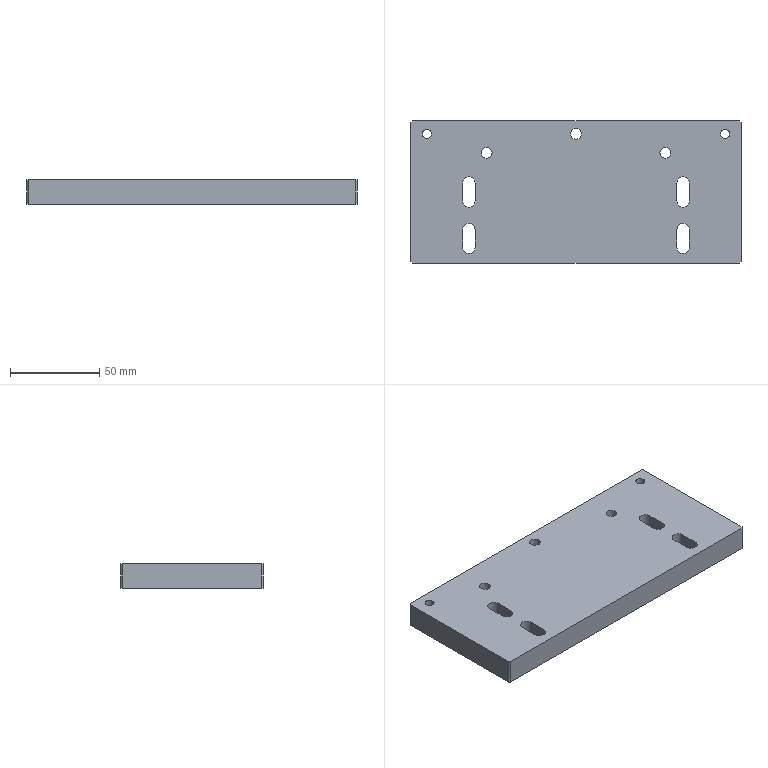CAM job | NX | 3-axis milling, drilling | part box 185 x 80 x 14 mm | stock box 190 x 85 x 20 mm
Tools:
number,name,description,diameter,corner_radius,flute_length,length,flutes
6,D6,平底铣刀-粗,6.0,0.0,25.0,75.0,2
9,D10,平底铣刀-粗,10.0,0.0,35.0,75.0,2
7,D6-J,平底铣刀-精,6.0,0.0,25.0,75.0,2
1,D80R0.8_FACEMILL,圆鼻刀-粗,80.0,0.8,50.0,75.0,2
1,D80R0.8_FACEMILL-J,圆鼻刀-精,80.0,0.8,50.0,75.0,2
2,D6_CHAMFERTOOL,倒角刀,6.0,0.0,3.0,25.0,2
22,M6X1.0,丝锥,5.0,0.0,35.0,50.0,2
18,D6_REAMER,Drilling Tool,6.0,0.0,75.0,100.0,6
15,ZT5.1,钻头,5.1,0.0,35.0,50.0,2
17,ZT5.9,Drilling Tool,5.9,0.0,35.0,50.0,2
Operations:
program,operation,operation_type,tool,method,geometry_group,spindle_rpm,surface_speed,feed_per_tooth,feed_cut,feed_plunge,cut_length_mm,path_length_mm,cut_time_min,machine_time_min
B,FLOORWALL_FACEROUGH_COPY,VolumeBased25DMillingOperation,D80R0.8_FACEMILL,LAYERED_ROUGH-DEPTHK-STEPG,W-B,2800.0,703.696,0.5357,3000.0,100.0,6343.672,6682.945,2.115,2.148
B,FLOORWALL_FACEFINISH_COPY,VolumeBased25DMillingOperation,D80R0.8_FACEMILL-J,SIDEWALL_FINISH-DEPTHK-STEPG,W-B,4000.0,1005.28,0.125,1000.0,100.0,576.11,672.11,0.5761,0.5857
B,MILL_CHAMFER_3,PlanarMilling,D6_CHAMFERTOOL,METHOD,W-B,8000.0,150.796,0.0375,600.0,100.0,37.911,408.52,0.0632,0.1002
B,PLANEDEBURR_6X45L_COPY,SurfaceContour,D6_CHAMFERTOOL,WALL_CHAMFER-DEPTH0-STEPG,W-B,6500.0,122.519,0.1154,1500.0,100.0,770.775,1450.944,0.5139,0.5819
A,TOPFACE,FaceMilling,D80R0.8_FACEMILL,SIDEWALL_FINISH-DEPTHK-STEPG,W-A,4500.0,1385.0,0.1667,1500.0,100.0,597.333,693.333,0.3982,0.4078
A,PROFILE_ROUGH_2,VolumeBased25DMillingOperation,D10,METHOD,W-A,8000.0,251.327,0.375,6000.0,80.0,11195.532,11308.032,1.866,1.877
A,SPOT-DEPTH0.8,Operation,D6_CHAMFERTOOL,NONE,W-A,8000.0,150.796,0.0312,500.0,90.0,9.0,294.443,0.018,0.0465
A,THRUHOLE-M6TAPDRILL,Operation,ZT5.1,NONE,W-A,2800.0,43.982,0.0625,350.0,90.0,46.0,360.003,0.1314,0.1628
A,THRUHOLE-FINE6.0_PREDRILL,Operation,ZT5.9,NONE,W-A,2500.0,46.339,0.05,250.0,90.0,59.109,322.42,0.2364,0.2628
A,THRUSLOT_ROUGH_1,VolumeBased25DMillingOperation,D6,METHOD,W-A,9000.0,169.646,0.1389,2500.0,100.0,6670.185,7294.295,2.668,2.731
A,SLOT_FINISH_1,VolumeBased25DMillingOperation,D6-J,METHOD,W-A,8000.0,150.796,0.0375,600.0,100.0,202.959,947.737,0.3383,0.4127
A,SELECTBODYONLY,SurfaceContour,D6_CHAMFERTOOL,METHOD,W-A,8000.0,150.796,0.1875,3000.0,100.0,716.837,1455.626,0.2389,0.3128
A,MILL_CHAMFER_1,PlanarMilling,D6_CHAMFERTOOL,METHOD,W-A,8000.0,150.796,0.0312,500.0,100.0,39.876,409.289,0.0798,0.1167
A,MILL_CHAMFER_2,PlanarMilling,D6_CHAMFERTOOL,METHOD,W-A,8000.0,150.796,0.0312,500.0,100.0,62.891,468.171,0.1258,0.1663
A,REAM_HOLE,Operation,D6_REAMER,METHOD,W-A,500.0,9.425,0.0167,50.0,0.0,48.0,300.201,0.96,0.9852
A,THRUHOLE-TAPM6,Operation,M6X1.0,METHOD,W-A,500.0,7.854,0.001,1.0,90.0,37.0,342.003,37.0,37.031
A,PROFILE_SEMIFINISH_2,VolumeBased25DMillingOperation,D6-J,METHOD,W-A,9000.0,169.646,0.0667,1200.0,100.0,1102.845,1345.366,0.919,0.9433